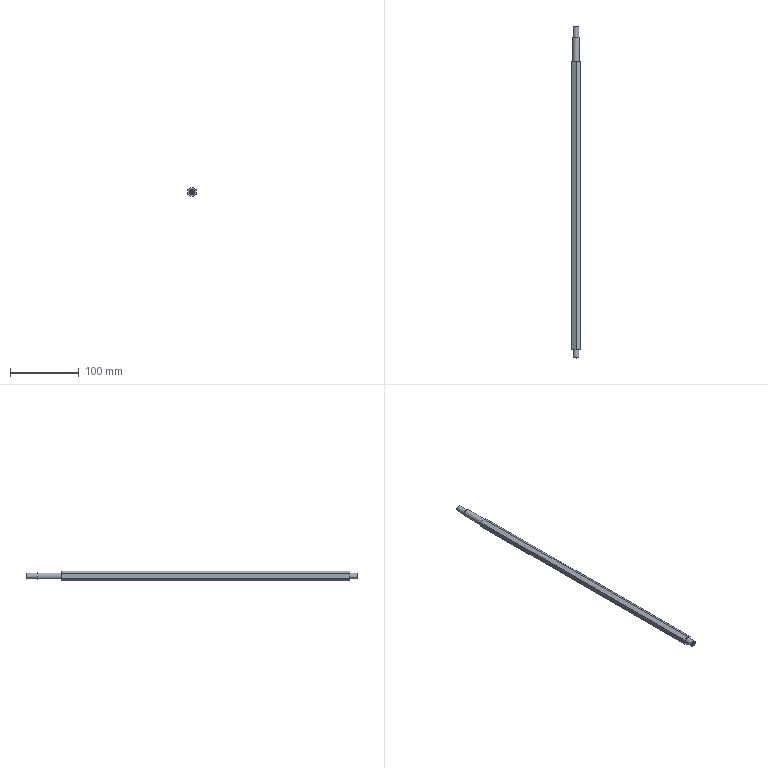Part | STEP file | ROTATION MC_NEW VER-0610_541 | 1 solid | 19 faces | box 12 x 481.5 x 13.856 mm | volume 56212 mm3 | plane 11 | cylinder 4 | cone 3 | torus 1 | commonest cylinder face diameters 8 x2 3.3 x1 10 x1
STEP:
#1=CARTESIAN_POINT('',(-236.469,227.468,-86.091));
#2=VERTEX_POINT('',#1);
#3=CARTESIAN_POINT('',(-228.469,227.468,-86.091));
#4=VERTEX_POINT('',#3);
#5=CARTESIAN_POINT('',(-232.469,227.468,-86.091));
#6=DIRECTION('',(0.,-1.,0.));
#7=DIRECTION('',(0.,0.,-1.));
#8=AXIS2_PLACEMENT_3D('',#5,#6,#7);
#9=CIRCLE('',#8,4.);
#10=EDGE_CURVE('',#2,#4,#9,.F.);
#11=ORIENTED_EDGE('',*,*,#10,.T.);
#12=CARTESIAN_POINT('',(-228.469,238.968,-86.091));
#13=VERTEX_POINT('',#12);
#14=CARTESIAN_POINT('',(-228.469,256.228,-86.091));
#15=DIRECTION('',(0.,1.,0.));
#16=VECTOR('',#15,4.);
#17=LINE('',#14,#16);
#18=EDGE_CURVE('',#4,#13,#17,.T.);
#19=ORIENTED_EDGE('',*,*,#18,.T.);
#20=CARTESIAN_POINT('',(-236.469,238.968,-86.091));
#21=VERTEX_POINT('',#20);
#22=CARTESIAN_POINT('',(-232.469,238.968,-86.091));
#23=DIRECTION('',(0.,-1.,0.));
#24=DIRECTION('',(0.,0.,-1.));
#25=AXIS2_PLACEMENT_3D('',#22,#23,#24);
#26=CIRCLE('',#25,4.);
#27=EDGE_CURVE('',#21,#13,#26,.F.);
#28=ORIENTED_EDGE('',*,*,#27,.F.);
#29=CARTESIAN_POINT('',(-232.469,238.968,-86.091));
#30=DIRECTION('',(0.,-1.,0.));
#31=DIRECTION('',(0.,0.,-1.));
#32=AXIS2_PLACEMENT_3D('',#29,#30,#31);
#33=CIRCLE('',#32,4.);
#34=EDGE_CURVE('',#13,#21,#33,.F.);
#35=ORIENTED_EDGE('',*,*,#34,.F.);
#36=ORIENTED_EDGE('',*,*,#18,.F.);
#37=CARTESIAN_POINT('',(-232.469,227.468,-90.091));
#38=VERTEX_POINT('',#37);
#39=CARTESIAN_POINT('',(-232.469,227.468,-86.091));
#40=DIRECTION('',(0.,-1.,0.));
#41=DIRECTION('',(0.,0.,-1.));
#42=AXIS2_PLACEMENT_3D('',#39,#40,#41);
#43=CIRCLE('',#42,4.);
#44=EDGE_CURVE('',#4,#38,#43,.F.);
#45=ORIENTED_EDGE('',*,*,#44,.T.);
#46=CARTESIAN_POINT('',(-232.469,227.468,-86.091));
#47=DIRECTION('',(0.,-1.,0.));
#48=DIRECTION('',(0.,0.,-1.));
#49=AXIS2_PLACEMENT_3D('',#46,#47,#48);
#50=CIRCLE('',#49,4.);
#51=EDGE_CURVE('',#38,#2,#50,.F.);
#52=ORIENTED_EDGE('',*,*,#51,.T.);
#53=EDGE_LOOP('',(#11,#19,#28,#35,#36,#45,#52));
#54=FACE_OUTER_BOUND('',#53,.T.);
#55=CARTESIAN_POINT('',(-232.469,256.228,-86.091));
#56=DIRECTION('',(0.,-1.,0.));
#57=DIRECTION('',(-1.,0.,0.));
#58=AXIS2_PLACEMENT_3D('',#55,#56,#57);
#59=CYLINDRICAL_SURFACE('',#58,4.);
#60=ADVANCED_FACE('',(#54),#59,.T.);
#61=CARTESIAN_POINT('',(-232.469,656.968,-80.891));
#62=VERTEX_POINT('',#61);
#63=CARTESIAN_POINT('',(-232.469,656.968,-86.091));
#64=DIRECTION('',(0.,-1.,0.));
#65=DIRECTION('',(0.,0.,1.));
#66=AXIS2_PLACEMENT_3D('',#63,#64,#65);
#67=CIRCLE('',#66,5.2);
#68=EDGE_CURVE('',#62,#62,#67,.T.);
#69=ORIENTED_EDGE('',*,*,#68,.F.);
#70=CARTESIAN_POINT('',(-232.469,657.168,-81.091));
#71=VERTEX_POINT('',#70);
#72=CARTESIAN_POINT('',(-232.469,657.168,-80.891));
#73=DIRECTION('',(1.,0.,0.));
#74=DIRECTION('',(0.,0.,1.));
#75=AXIS2_PLACEMENT_3D('',#72,#73,#74);
#76=CIRCLE('',#75,0.2);
#77=EDGE_CURVE('',#62,#71,#76,.T.);
#78=ORIENTED_EDGE('',*,*,#77,.T.);
#79=CARTESIAN_POINT('',(-237.469,657.168,-86.091));
#80=VERTEX_POINT('',#79);
#81=CARTESIAN_POINT('',(-232.469,657.168,-86.091));
#82=DIRECTION('',(0.,1.,0.));
#83=DIRECTION('',(0.,0.,1.));
#84=AXIS2_PLACEMENT_3D('',#81,#82,#83);
#85=CIRCLE('',#84,5.);
#86=EDGE_CURVE('',#80,#71,#85,.T.);
#87=ORIENTED_EDGE('',*,*,#86,.F.);
#88=CARTESIAN_POINT('',(-232.469,657.168,-86.091));
#89=DIRECTION('',(0.,1.,0.));
#90=DIRECTION('',(0.,0.,1.));
#91=AXIS2_PLACEMENT_3D('',#88,#89,#90);
#92=CIRCLE('',#91,5.);
#93=EDGE_CURVE('',#71,#80,#92,.T.);
#94=ORIENTED_EDGE('',*,*,#93,.F.);
#95=ORIENTED_EDGE('',*,*,#77,.F.);
#96=EDGE_LOOP('',(#69,#78,#87,#94,#95));
#97=FACE_OUTER_BOUND('',#96,.T.);
#98=CARTESIAN_POINT('',(-232.469,657.168,-86.091));
#99=DIRECTION('',(0.,-1.,0.));
#100=DIRECTION('',(0.,0.,-1.));
#101=AXIS2_PLACEMENT_3D('',#98,#99,#100);
#102=TOROIDAL_SURFACE('',#101,5.2,0.2);
#103=ADVANCED_FACE('',(#97),#102,.F.);
#104=CARTESIAN_POINT('',(-238.469,238.968,-82.627));
#105=VERTEX_POINT('',#104);
#106=CARTESIAN_POINT('',(-232.469,238.968,-79.163));
#107=VERTEX_POINT('',#106);
#108=CARTESIAN_POINT('',(-238.469,238.968,-82.627));
#109=DIRECTION('',(0.866,0.,0.5));
#110=VECTOR('',#109,6.928);
#111=LINE('',#108,#110);
#112=EDGE_CURVE('',#105,#107,#111,.T.);
#113=ORIENTED_EDGE('',*,*,#112,.T.);
#114=CARTESIAN_POINT('',(-232.469,656.968,-79.163));
#115=VERTEX_POINT('',#114);
#116=CARTESIAN_POINT('',(-232.469,238.968,-79.163));
#117=DIRECTION('',(0.,1.,0.));
#118=VECTOR('',#117,418.);
#119=LINE('',#116,#118);
#120=EDGE_CURVE('',#107,#115,#119,.T.);
#121=ORIENTED_EDGE('',*,*,#120,.T.);
#122=CARTESIAN_POINT('',(-238.469,656.968,-82.627));
#123=VERTEX_POINT('',#122);
#124=CARTESIAN_POINT('',(-232.469,656.968,-79.163));
#125=DIRECTION('',(-0.866,0.,-0.5));
#126=VECTOR('',#125,6.928);
#127=LINE('',#124,#126);
#128=EDGE_CURVE('',#115,#123,#127,.T.);
#129=ORIENTED_EDGE('',*,*,#128,.T.);
#130=CARTESIAN_POINT('',(-238.469,238.968,-82.627));
#131=DIRECTION('',(0.,1.,0.));
#132=VECTOR('',#131,418.);
#133=LINE('',#130,#132);
#134=EDGE_CURVE('',#105,#123,#133,.T.);
#135=ORIENTED_EDGE('',*,*,#134,.F.);
#136=EDGE_LOOP('',(#113,#121,#129,#135));
#137=FACE_OUTER_BOUND('',#136,.T.);
#138=CARTESIAN_POINT('',(-235.469,583.228,-80.895));
#139=DIRECTION('',(-0.5,0.,0.866));
#140=DIRECTION('',(0.866,0.,0.5));
#141=AXIS2_PLACEMENT_3D('',#138,#139,#140);
#142=PLANE('',#141);
#143=ADVANCED_FACE('',(#137),#142,.T.);
#144=CARTESIAN_POINT('',(-238.469,656.968,-89.555));
#145=VERTEX_POINT('',#144);
#146=CARTESIAN_POINT('',(-238.469,656.968,-82.627));
#147=DIRECTION('',(0.,0.,-1.));
#148=VECTOR('',#147,6.928);
#149=LINE('',#146,#148);
#150=EDGE_CURVE('',#123,#145,#149,.T.);
#151=ORIENTED_EDGE('',*,*,#150,.T.);
#152=CARTESIAN_POINT('',(-238.469,238.968,-89.555));
#153=VERTEX_POINT('',#152);
#154=CARTESIAN_POINT('',(-238.469,238.968,-89.555));
#155=DIRECTION('',(0.,1.,0.));
#156=VECTOR('',#155,418.);
#157=LINE('',#154,#156);
#158=EDGE_CURVE('',#153,#145,#157,.T.);
#159=ORIENTED_EDGE('',*,*,#158,.F.);
#160=CARTESIAN_POINT('',(-238.469,238.968,-89.555));
#161=DIRECTION('',(0.,0.,1.));
#162=VECTOR('',#161,6.928);
#163=LINE('',#160,#162);
#164=EDGE_CURVE('',#153,#105,#163,.T.);
#165=ORIENTED_EDGE('',*,*,#164,.T.);
#166=ORIENTED_EDGE('',*,*,#134,.T.);
#167=EDGE_LOOP('',(#151,#159,#165,#166));
#168=FACE_OUTER_BOUND('',#167,.T.);
#169=CARTESIAN_POINT('',(-238.469,583.228,-86.091));
#170=DIRECTION('',(-1.,0.,0.));
#171=DIRECTION('',(0.,0.,1.));
#172=AXIS2_PLACEMENT_3D('',#169,#170,#171);
#173=PLANE('',#172);
#174=ADVANCED_FACE('',(#168),#173,.T.);
#175=ORIENTED_EDGE('',*,*,#128,.F.);
#176=CARTESIAN_POINT('',(-226.469,656.968,-82.627));
#177=VERTEX_POINT('',#176);
#178=CARTESIAN_POINT('',(-226.469,656.968,-82.627));
#179=DIRECTION('',(-0.866,0.,0.5));
#180=VECTOR('',#179,6.928);
#181=LINE('',#178,#180);
#182=EDGE_CURVE('',#177,#115,#181,.T.);
#183=ORIENTED_EDGE('',*,*,#182,.F.);
#184=CARTESIAN_POINT('',(-226.469,656.968,-89.555));
#185=VERTEX_POINT('',#184);
#186=CARTESIAN_POINT('',(-226.469,656.968,-89.555));
#187=DIRECTION('',(0.,0.,1.));
#188=VECTOR('',#187,6.928);
#189=LINE('',#186,#188);
#190=EDGE_CURVE('',#185,#177,#189,.T.);
#191=ORIENTED_EDGE('',*,*,#190,.F.);
#192=CARTESIAN_POINT('',(-232.469,656.968,-93.019));
#193=VERTEX_POINT('',#192);
#194=CARTESIAN_POINT('',(-232.469,656.968,-93.019));
#195=DIRECTION('',(0.866,0.,0.5));
#196=VECTOR('',#195,6.928);
#197=LINE('',#194,#196);
#198=EDGE_CURVE('',#193,#185,#197,.T.);
#199=ORIENTED_EDGE('',*,*,#198,.F.);
#200=CARTESIAN_POINT('',(-238.469,656.968,-89.555));
#201=DIRECTION('',(0.866,0.,-0.5));
#202=VECTOR('',#201,6.928);
#203=LINE('',#200,#202);
#204=EDGE_CURVE('',#145,#193,#203,.T.);
#205=ORIENTED_EDGE('',*,*,#204,.F.);
#206=ORIENTED_EDGE('',*,*,#150,.F.);
#207=EDGE_LOOP('',(#175,#183,#191,#199,#205,#206));
#208=FACE_OUTER_BOUND('',#207,.T.);
#209=ORIENTED_EDGE('',*,*,#68,.T.);
#210=EDGE_LOOP('',(#209));
#211=FACE_BOUND('',#210,.T.);
#212=CARTESIAN_POINT('',(-233.469,656.968,-56.281));
#213=DIRECTION('',(0.,-1.,0.));
#214=DIRECTION('',(0.,0.,-1.));
#215=AXIS2_PLACEMENT_3D('',#212,#213,#214);
#216=PLANE('',#215);
#217=ADVANCED_FACE('',(#208,#211),#216,.F.);
#218=ORIENTED_EDGE('',*,*,#190,.T.);
#219=CARTESIAN_POINT('',(-226.469,238.968,-82.627));
#220=VERTEX_POINT('',#219);
#221=CARTESIAN_POINT('',(-226.469,238.968,-82.627));
#222=DIRECTION('',(0.,1.,0.));
#223=VECTOR('',#222,418.);
#224=LINE('',#221,#223);
#225=EDGE_CURVE('',#220,#177,#224,.T.);
#226=ORIENTED_EDGE('',*,*,#225,.F.);
#227=CARTESIAN_POINT('',(-226.469,238.968,-89.555));
#228=VERTEX_POINT('',#227);
#229=CARTESIAN_POINT('',(-226.469,238.968,-82.627));
#230=DIRECTION('',(0.,0.,-1.));
#231=VECTOR('',#230,6.928);
#232=LINE('',#229,#231);
#233=EDGE_CURVE('',#220,#228,#232,.T.);
#234=ORIENTED_EDGE('',*,*,#233,.T.);
#235=CARTESIAN_POINT('',(-226.469,238.968,-89.555));
#236=DIRECTION('',(0.,1.,0.));
#237=VECTOR('',#236,418.);
#238=LINE('',#235,#237);
#239=EDGE_CURVE('',#228,#185,#238,.T.);
#240=ORIENTED_EDGE('',*,*,#239,.T.);
#241=EDGE_LOOP('',(#218,#226,#234,#240));
#242=FACE_OUTER_BOUND('',#241,.T.);
#243=CARTESIAN_POINT('',(-226.469,583.228,-86.091));
#244=DIRECTION('',(1.,0.,0.));
#245=DIRECTION('',(0.,0.,-1.));
#246=AXIS2_PLACEMENT_3D('',#243,#244,#245);
#247=PLANE('',#246);
#248=ADVANCED_FACE('',(#242),#247,.T.);
#249=ORIENTED_EDGE('',*,*,#204,.T.);
#250=CARTESIAN_POINT('',(-232.469,238.968,-93.019));
#251=VERTEX_POINT('',#250);
#252=CARTESIAN_POINT('',(-232.469,238.968,-93.019));
#253=DIRECTION('',(0.,1.,0.));
#254=VECTOR('',#253,418.);
#255=LINE('',#252,#254);
#256=EDGE_CURVE('',#251,#193,#255,.T.);
#257=ORIENTED_EDGE('',*,*,#256,.F.);
#258=CARTESIAN_POINT('',(-232.469,238.968,-93.019));
#259=DIRECTION('',(-0.866,0.,0.5));
#260=VECTOR('',#259,6.928);
#261=LINE('',#258,#260);
#262=EDGE_CURVE('',#251,#153,#261,.T.);
#263=ORIENTED_EDGE('',*,*,#262,.T.);
#264=ORIENTED_EDGE('',*,*,#158,.T.);
#265=EDGE_LOOP('',(#249,#257,#263,#264));
#266=FACE_OUTER_BOUND('',#265,.T.);
#267=CARTESIAN_POINT('',(-235.469,583.228,-91.287));
#268=DIRECTION('',(-0.5,0.,-0.866));
#269=DIRECTION('',(-0.866,0.,0.5));
#270=AXIS2_PLACEMENT_3D('',#267,#268,#269);
#271=PLANE('',#270);
#272=ADVANCED_FACE('',(#266),#271,.T.);
#273=ORIENTED_EDGE('',*,*,#198,.T.);
#274=ORIENTED_EDGE('',*,*,#239,.F.);
#275=CARTESIAN_POINT('',(-226.469,238.968,-89.555));
#276=DIRECTION('',(-0.866,0.,-0.5));
#277=VECTOR('',#276,6.928);
#278=LINE('',#275,#277);
#279=EDGE_CURVE('',#228,#251,#278,.T.);
#280=ORIENTED_EDGE('',*,*,#279,.T.);
#281=ORIENTED_EDGE('',*,*,#256,.T.);
#282=EDGE_LOOP('',(#273,#274,#280,#281));
#283=FACE_OUTER_BOUND('',#282,.T.);
#284=CARTESIAN_POINT('',(-229.469,583.228,-91.287));
#285=DIRECTION('',(0.5,0.,-0.866));
#286=DIRECTION('',(-0.866,0.,-0.5));
#287=AXIS2_PLACEMENT_3D('',#284,#285,#286);
#288=PLANE('',#287);
#289=ADVANCED_FACE('',(#283),#288,.T.);
#290=CARTESIAN_POINT('',(-228.969,708.468,-86.091));
#291=VERTEX_POINT('',#290);
#292=CARTESIAN_POINT('',(-232.469,708.468,-86.091));
#293=DIRECTION('',(0.,-1.,0.));
#294=DIRECTION('',(1.,0.,0.));
#295=AXIS2_PLACEMENT_3D('',#292,#293,#294);
#296=CIRCLE('',#295,3.5);
#297=EDGE_CURVE('',#291,#291,#296,.T.);
#298=ORIENTED_EDGE('',*,*,#297,.F.);
#299=EDGE_LOOP('',(#298));
#300=FACE_OUTER_BOUND('',#299,.T.);
#301=CARTESIAN_POINT('',(-232.469,708.468,-86.091));
#302=DIRECTION('',(0.,1.,0.));
#303=DIRECTION('',(0.,0.,1.));
#304=AXIS2_PLACEMENT_3D('',#301,#302,#303);
#305=PLANE('',#304);
#306=ADVANCED_FACE('',(#300),#305,.T.);
#307=ORIENTED_EDGE('',*,*,#182,.T.);
#308=ORIENTED_EDGE('',*,*,#120,.F.);
#309=CARTESIAN_POINT('',(-232.469,238.968,-79.163));
#310=DIRECTION('',(0.866,0.,-0.5));
#311=VECTOR('',#310,6.928);
#312=LINE('',#309,#311);
#313=EDGE_CURVE('',#107,#220,#312,.T.);
#314=ORIENTED_EDGE('',*,*,#313,.T.);
#315=ORIENTED_EDGE('',*,*,#225,.T.);
#316=EDGE_LOOP('',(#307,#308,#314,#315));
#317=FACE_OUTER_BOUND('',#316,.T.);
#318=CARTESIAN_POINT('',(-229.469,583.228,-80.895));
#319=DIRECTION('',(0.5,0.,0.866));
#320=DIRECTION('',(0.866,0.,-0.5));
#321=AXIS2_PLACEMENT_3D('',#318,#319,#320);
#322=PLANE('',#321);
#323=ADVANCED_FACE('',(#317),#322,.T.);
#324=ORIENTED_EDGE('',*,*,#164,.F.);
#325=ORIENTED_EDGE('',*,*,#262,.F.);
#326=ORIENTED_EDGE('',*,*,#279,.F.);
#327=ORIENTED_EDGE('',*,*,#233,.F.);
#328=ORIENTED_EDGE('',*,*,#313,.F.);
#329=ORIENTED_EDGE('',*,*,#112,.F.);
#330=EDGE_LOOP('',(#324,#325,#326,#327,#328,#329));
#331=FACE_OUTER_BOUND('',#330,.T.);
#332=ORIENTED_EDGE('',*,*,#27,.T.);
#333=ORIENTED_EDGE('',*,*,#34,.T.);
#334=EDGE_LOOP('',(#332,#333));
#335=FACE_BOUND('',#334,.T.);
#336=CARTESIAN_POINT('',(-233.469,238.968,-56.281));
#337=DIRECTION('',(0.,-1.,0.));
#338=DIRECTION('',(0.,0.,-1.));
#339=AXIS2_PLACEMENT_3D('',#336,#337,#338);
#340=PLANE('',#339);
#341=ADVANCED_FACE('',(#331,#335),#340,.T.);
#342=CARTESIAN_POINT('',(-237.469,692.468,-86.091));
#343=VERTEX_POINT('',#342);
#344=CARTESIAN_POINT('',(-232.469,692.468,-86.091));
#345=DIRECTION('',(0.,1.,0.));
#346=DIRECTION('',(-1.,0.,0.));
#347=AXIS2_PLACEMENT_3D('',#344,#345,#346);
#348=CIRCLE('',#347,5.);
#349=EDGE_CURVE('',#343,#343,#348,.T.);
#350=ORIENTED_EDGE('',*,*,#349,.F.);
#351=CARTESIAN_POINT('',(-237.469,708.228,-86.091));
#352=DIRECTION('',(0.,-1.,0.));
#353=VECTOR('',#352,5.);
#354=LINE('',#351,#353);
#355=EDGE_CURVE('',#343,#80,#354,.T.);
#356=ORIENTED_EDGE('',*,*,#355,.T.);
#357=ORIENTED_EDGE('',*,*,#86,.T.);
#358=ORIENTED_EDGE('',*,*,#93,.T.);
#359=ORIENTED_EDGE('',*,*,#355,.F.);
#360=EDGE_LOOP('',(#350,#356,#357,#358,#359));
#361=FACE_OUTER_BOUND('',#360,.T.);
#362=CARTESIAN_POINT('',(-232.469,708.228,-86.091));
#363=DIRECTION('',(0.,1.,0.));
#364=DIRECTION('',(1.,0.,0.));
#365=AXIS2_PLACEMENT_3D('',#362,#363,#364);
#366=CYLINDRICAL_SURFACE('',#365,5.);
#367=ADVANCED_FACE('',(#361),#366,.T.);
#368=CARTESIAN_POINT('',(-236.469,707.968,-86.091));
#369=VERTEX_POINT('',#368);
#370=CARTESIAN_POINT('',(-228.469,707.968,-86.091));
#371=VERTEX_POINT('',#370);
#372=CARTESIAN_POINT('',(-232.469,707.968,-86.091));
#373=DIRECTION('',(0.,1.,0.));
#374=DIRECTION('',(1.,0.,0.));
#375=AXIS2_PLACEMENT_3D('',#372,#373,#374);
#376=CIRCLE('',#375,4.);
#377=EDGE_CURVE('',#369,#371,#376,.T.);
#378=ORIENTED_EDGE('',*,*,#377,.T.);
#379=CARTESIAN_POINT('',(-228.969,708.468,-86.091));
#380=DIRECTION('',(-0.7071,0.7071,0.));
#381=VECTOR('',#380,3.5);
#382=LINE('',#379,#381);
#383=EDGE_CURVE('',#371,#291,#382,.T.);
#384=ORIENTED_EDGE('',*,*,#383,.T.);
#385=ORIENTED_EDGE('',*,*,#297,.T.);
#386=ORIENTED_EDGE('',*,*,#383,.F.);
#387=CARTESIAN_POINT('',(-232.469,707.968,-86.091));
#388=DIRECTION('',(0.,1.,0.));
#389=DIRECTION('',(1.,0.,0.));
#390=AXIS2_PLACEMENT_3D('',#387,#388,#389);
#391=CIRCLE('',#390,4.);
#392=EDGE_CURVE('',#371,#369,#391,.T.);
#393=ORIENTED_EDGE('',*,*,#392,.T.);
#394=EDGE_LOOP('',(#378,#384,#385,#386,#393));
#395=FACE_OUTER_BOUND('',#394,.T.);
#396=CARTESIAN_POINT('',(-232.469,708.468,-86.091));
#397=DIRECTION('',(0.,-1.,0.));
#398=DIRECTION('',(-1.,0.,0.));
#399=AXIS2_PLACEMENT_3D('',#396,#397,#398);
#400=CONICAL_SURFACE('',#399,3.5,0.7854);
#401=ADVANCED_FACE('',(#395),#400,.T.);
#402=ORIENTED_EDGE('',*,*,#349,.T.);
#403=EDGE_LOOP('',(#402));
#404=FACE_OUTER_BOUND('',#403,.T.);
#405=CARTESIAN_POINT('',(-236.469,692.468,-86.091));
#406=VERTEX_POINT('',#405);
#407=CARTESIAN_POINT('',(-232.469,692.468,-86.091));
#408=DIRECTION('',(0.,-1.,0.));
#409=DIRECTION('',(1.,0.,0.));
#410=AXIS2_PLACEMENT_3D('',#407,#408,#409);
#411=CIRCLE('',#410,4.);
#412=EDGE_CURVE('',#406,#406,#411,.T.);
#413=ORIENTED_EDGE('',*,*,#412,.T.);
#414=EDGE_LOOP('',(#413));
#415=FACE_BOUND('',#414,.T.);
#416=CARTESIAN_POINT('',(-244.469,692.468,-86.091));
#417=DIRECTION('',(0.,-1.,0.));
#418=DIRECTION('',(0.,0.,-1.));
#419=AXIS2_PLACEMENT_3D('',#416,#417,#418);
#420=PLANE('',#419);
#421=ADVANCED_FACE('',(#404,#415),#420,.F.);
#422=ORIENTED_EDGE('',*,*,#377,.F.);
#423=CARTESIAN_POINT('',(-236.469,708.228,-86.091));
#424=DIRECTION('',(0.,-1.,0.));
#425=VECTOR('',#424,4.);
#426=LINE('',#423,#425);
#427=EDGE_CURVE('',#369,#406,#426,.T.);
#428=ORIENTED_EDGE('',*,*,#427,.T.);
#429=ORIENTED_EDGE('',*,*,#412,.F.);
#430=ORIENTED_EDGE('',*,*,#427,.F.);
#431=ORIENTED_EDGE('',*,*,#392,.F.);
#432=EDGE_LOOP('',(#422,#428,#429,#430,#431));
#433=FACE_OUTER_BOUND('',#432,.T.);
#434=CARTESIAN_POINT('',(-232.469,708.228,-86.091));
#435=DIRECTION('',(0.,1.,0.));
#436=DIRECTION('',(1.,0.,0.));
#437=AXIS2_PLACEMENT_3D('',#434,#435,#436);
#438=CYLINDRICAL_SURFACE('',#437,4.);
#439=ADVANCED_FACE('',(#433),#438,.T.);
#440=CARTESIAN_POINT('',(-235.969,226.968,-86.091));
#441=VERTEX_POINT('',#440);
#442=CARTESIAN_POINT('',(-232.469,226.968,-89.591));
#443=VERTEX_POINT('',#442);
#444=CARTESIAN_POINT('',(-232.469,226.968,-86.091));
#445=DIRECTION('',(0.,-1.,0.));
#446=DIRECTION('',(1.,0.,0.));
#447=AXIS2_PLACEMENT_3D('',#444,#445,#446);
#448=CIRCLE('',#447,3.5);
#449=EDGE_CURVE('',#441,#443,#448,.T.);
#450=ORIENTED_EDGE('',*,*,#449,.T.);
#451=CARTESIAN_POINT('',(-232.469,226.968,-86.091));
#452=DIRECTION('',(0.,-1.,0.));
#453=DIRECTION('',(1.,0.,0.));
#454=AXIS2_PLACEMENT_3D('',#451,#452,#453);
#455=CIRCLE('',#454,3.5);
#456=EDGE_CURVE('',#443,#441,#455,.T.);
#457=ORIENTED_EDGE('',*,*,#456,.T.);
#458=EDGE_LOOP('',(#450,#457));
#459=FACE_OUTER_BOUND('',#458,.T.);
#460=CARTESIAN_POINT('',(-234.119,226.968,-86.091));
#461=VERTEX_POINT('',#460);
#462=CARTESIAN_POINT('',(-230.819,226.968,-86.091));
#463=VERTEX_POINT('',#462);
#464=CARTESIAN_POINT('',(-232.469,226.968,-86.091));
#465=DIRECTION('',(0.,1.,0.));
#466=DIRECTION('',(-1.,0.,0.));
#467=AXIS2_PLACEMENT_3D('',#464,#465,#466);
#468=CIRCLE('',#467,1.65);
#469=EDGE_CURVE('',#461,#463,#468,.T.);
#470=ORIENTED_EDGE('',*,*,#469,.T.);
#471=CARTESIAN_POINT('',(-232.469,226.968,-86.091));
#472=DIRECTION('',(0.,1.,0.));
#473=DIRECTION('',(-1.,0.,0.));
#474=AXIS2_PLACEMENT_3D('',#471,#472,#473);
#475=CIRCLE('',#474,1.65);
#476=EDGE_CURVE('',#463,#461,#475,.T.);
#477=ORIENTED_EDGE('',*,*,#476,.T.);
#478=EDGE_LOOP('',(#470,#477));
#479=FACE_BOUND('',#478,.T.);
#480=CARTESIAN_POINT('',(-279.969,226.968,-96.341));
#481=DIRECTION('',(0.,-1.,0.));
#482=DIRECTION('',(0.,0.,-1.));
#483=AXIS2_PLACEMENT_3D('',#480,#481,#482);
#484=PLANE('',#483);
#485=ADVANCED_FACE('',(#459,#479),#484,.T.);
#486=CARTESIAN_POINT('',(-232.469,239.96,-86.091));
#487=VERTEX_POINT('',#486);
#488=CARTESIAN_POINT('',(-234.119,238.968,-86.091));
#489=VERTEX_POINT('',#488);
#490=CARTESIAN_POINT('',(-234.119,238.968,-86.091));
#491=DIRECTION('',(-0.8572,-0.515,0.));
#492=VECTOR('',#491,1.65);
#493=LINE('',#490,#492);
#494=EDGE_CURVE('',#487,#489,#493,.T.);
#495=ORIENTED_EDGE('',*,*,#494,.T.);
#496=CARTESIAN_POINT('',(-230.819,238.968,-86.091));
#497=VERTEX_POINT('',#496);
#498=CARTESIAN_POINT('',(-232.469,238.968,-86.091));
#499=DIRECTION('',(0.,1.,0.));
#500=DIRECTION('',(-1.,0.,0.));
#501=AXIS2_PLACEMENT_3D('',#498,#499,#500);
#502=CIRCLE('',#501,1.65);
#503=EDGE_CURVE('',#489,#497,#502,.F.);
#504=ORIENTED_EDGE('',*,*,#503,.T.);
#505=CARTESIAN_POINT('',(-232.469,238.968,-86.091));
#506=DIRECTION('',(0.,1.,0.));
#507=DIRECTION('',(-1.,0.,0.));
#508=AXIS2_PLACEMENT_3D('',#505,#506,#507);
#509=CIRCLE('',#508,1.65);
#510=EDGE_CURVE('',#497,#489,#509,.F.);
#511=ORIENTED_EDGE('',*,*,#510,.T.);
#512=ORIENTED_EDGE('',*,*,#494,.F.);
#513=EDGE_LOOP('',(#495,#504,#511,#512));
#514=FACE_OUTER_BOUND('',#513,.T.);
#515=CARTESIAN_POINT('',(-232.469,238.968,-86.091));
#516=DIRECTION('',(0.,-1.,0.));
#517=DIRECTION('',(1.,0.,0.));
#518=AXIS2_PLACEMENT_3D('',#515,#516,#517);
#519=CONICAL_SURFACE('',#518,1.65,1.03);
#520=ADVANCED_FACE('',(#514),#519,.F.);
#521=ORIENTED_EDGE('',*,*,#469,.F.);
#522=ORIENTED_EDGE('',*,*,#476,.F.);
#523=CARTESIAN_POINT('',(-230.819,226.968,-86.091));
#524=DIRECTION('',(0.,1.,0.));
#525=VECTOR('',#524,1.65);
#526=LINE('',#523,#525);
#527=EDGE_CURVE('',#463,#497,#526,.T.);
#528=ORIENTED_EDGE('',*,*,#527,.T.);
#529=ORIENTED_EDGE('',*,*,#503,.F.);
#530=ORIENTED_EDGE('',*,*,#510,.F.);
#531=ORIENTED_EDGE('',*,*,#527,.F.);
#532=EDGE_LOOP('',(#521,#522,#528,#529,#530,#531));
#533=FACE_OUTER_BOUND('',#532,.T.);
#534=CARTESIAN_POINT('',(-232.469,226.968,-86.091));
#535=DIRECTION('',(0.,1.,0.));
#536=DIRECTION('',(-1.,0.,0.));
#537=AXIS2_PLACEMENT_3D('',#534,#535,#536);
#538=CYLINDRICAL_SURFACE('',#537,1.65);
#539=ADVANCED_FACE('',(#533),#538,.F.);
#540=ORIENTED_EDGE('',*,*,#10,.F.);
#541=ORIENTED_EDGE('',*,*,#51,.F.);
#542=CARTESIAN_POINT('',(-232.469,227.468,-90.091));
#543=DIRECTION('',(0.,-0.7071,0.7071));
#544=VECTOR('',#543,4.);
#545=LINE('',#542,#544);
#546=EDGE_CURVE('',#38,#443,#545,.T.);
#547=ORIENTED_EDGE('',*,*,#546,.T.);
#548=ORIENTED_EDGE('',*,*,#449,.F.);
#549=ORIENTED_EDGE('',*,*,#456,.F.);
#550=ORIENTED_EDGE('',*,*,#546,.F.);
#551=ORIENTED_EDGE('',*,*,#44,.F.);
#552=EDGE_LOOP('',(#540,#541,#547,#548,#549,#550,#551));
#553=FACE_OUTER_BOUND('',#552,.T.);
#554=CARTESIAN_POINT('',(-232.469,227.468,-86.091));
#555=DIRECTION('',(0.,1.,0.));
#556=DIRECTION('',(0.,0.,1.));
#557=AXIS2_PLACEMENT_3D('',#554,#555,#556);
#558=CONICAL_SURFACE('',#557,4.,0.7854);
#559=ADVANCED_FACE('',(#553),#558,.T.);
#560=CLOSED_SHELL('',(#60,#103,#143,#174,#217,#248,#272,#289,#306,#323,#341,#367,#401,#421,#439,#485,#520,#539,#559));
#561=MANIFOLD_SOLID_BREP('',#560);
#562=(LENGTH_UNIT()NAMED_UNIT(*)SI_UNIT(.MILLI.,.METRE.));
#563=UNCERTAINTY_MEASURE_WITH_UNIT(LENGTH_MEASURE(0.01),#562,'','');
#564=(NAMED_UNIT(*)PLANE_ANGLE_UNIT()SI_UNIT($,.RADIAN.));
#565=(NAMED_UNIT(*)SI_UNIT($,.STERADIAN.)SOLID_ANGLE_UNIT());
#566=(GEOMETRIC_REPRESENTATION_CONTEXT(3)GLOBAL_UNCERTAINTY_ASSIGNED_CONTEXT((#563))GLOBAL_UNIT_ASSIGNED_CONTEXT((#562,#564,#565))REPRESENTATION_CONTEXT('',''));
#567=ADVANCED_BREP_SHAPE_REPRESENTATION('',(#561),#566);